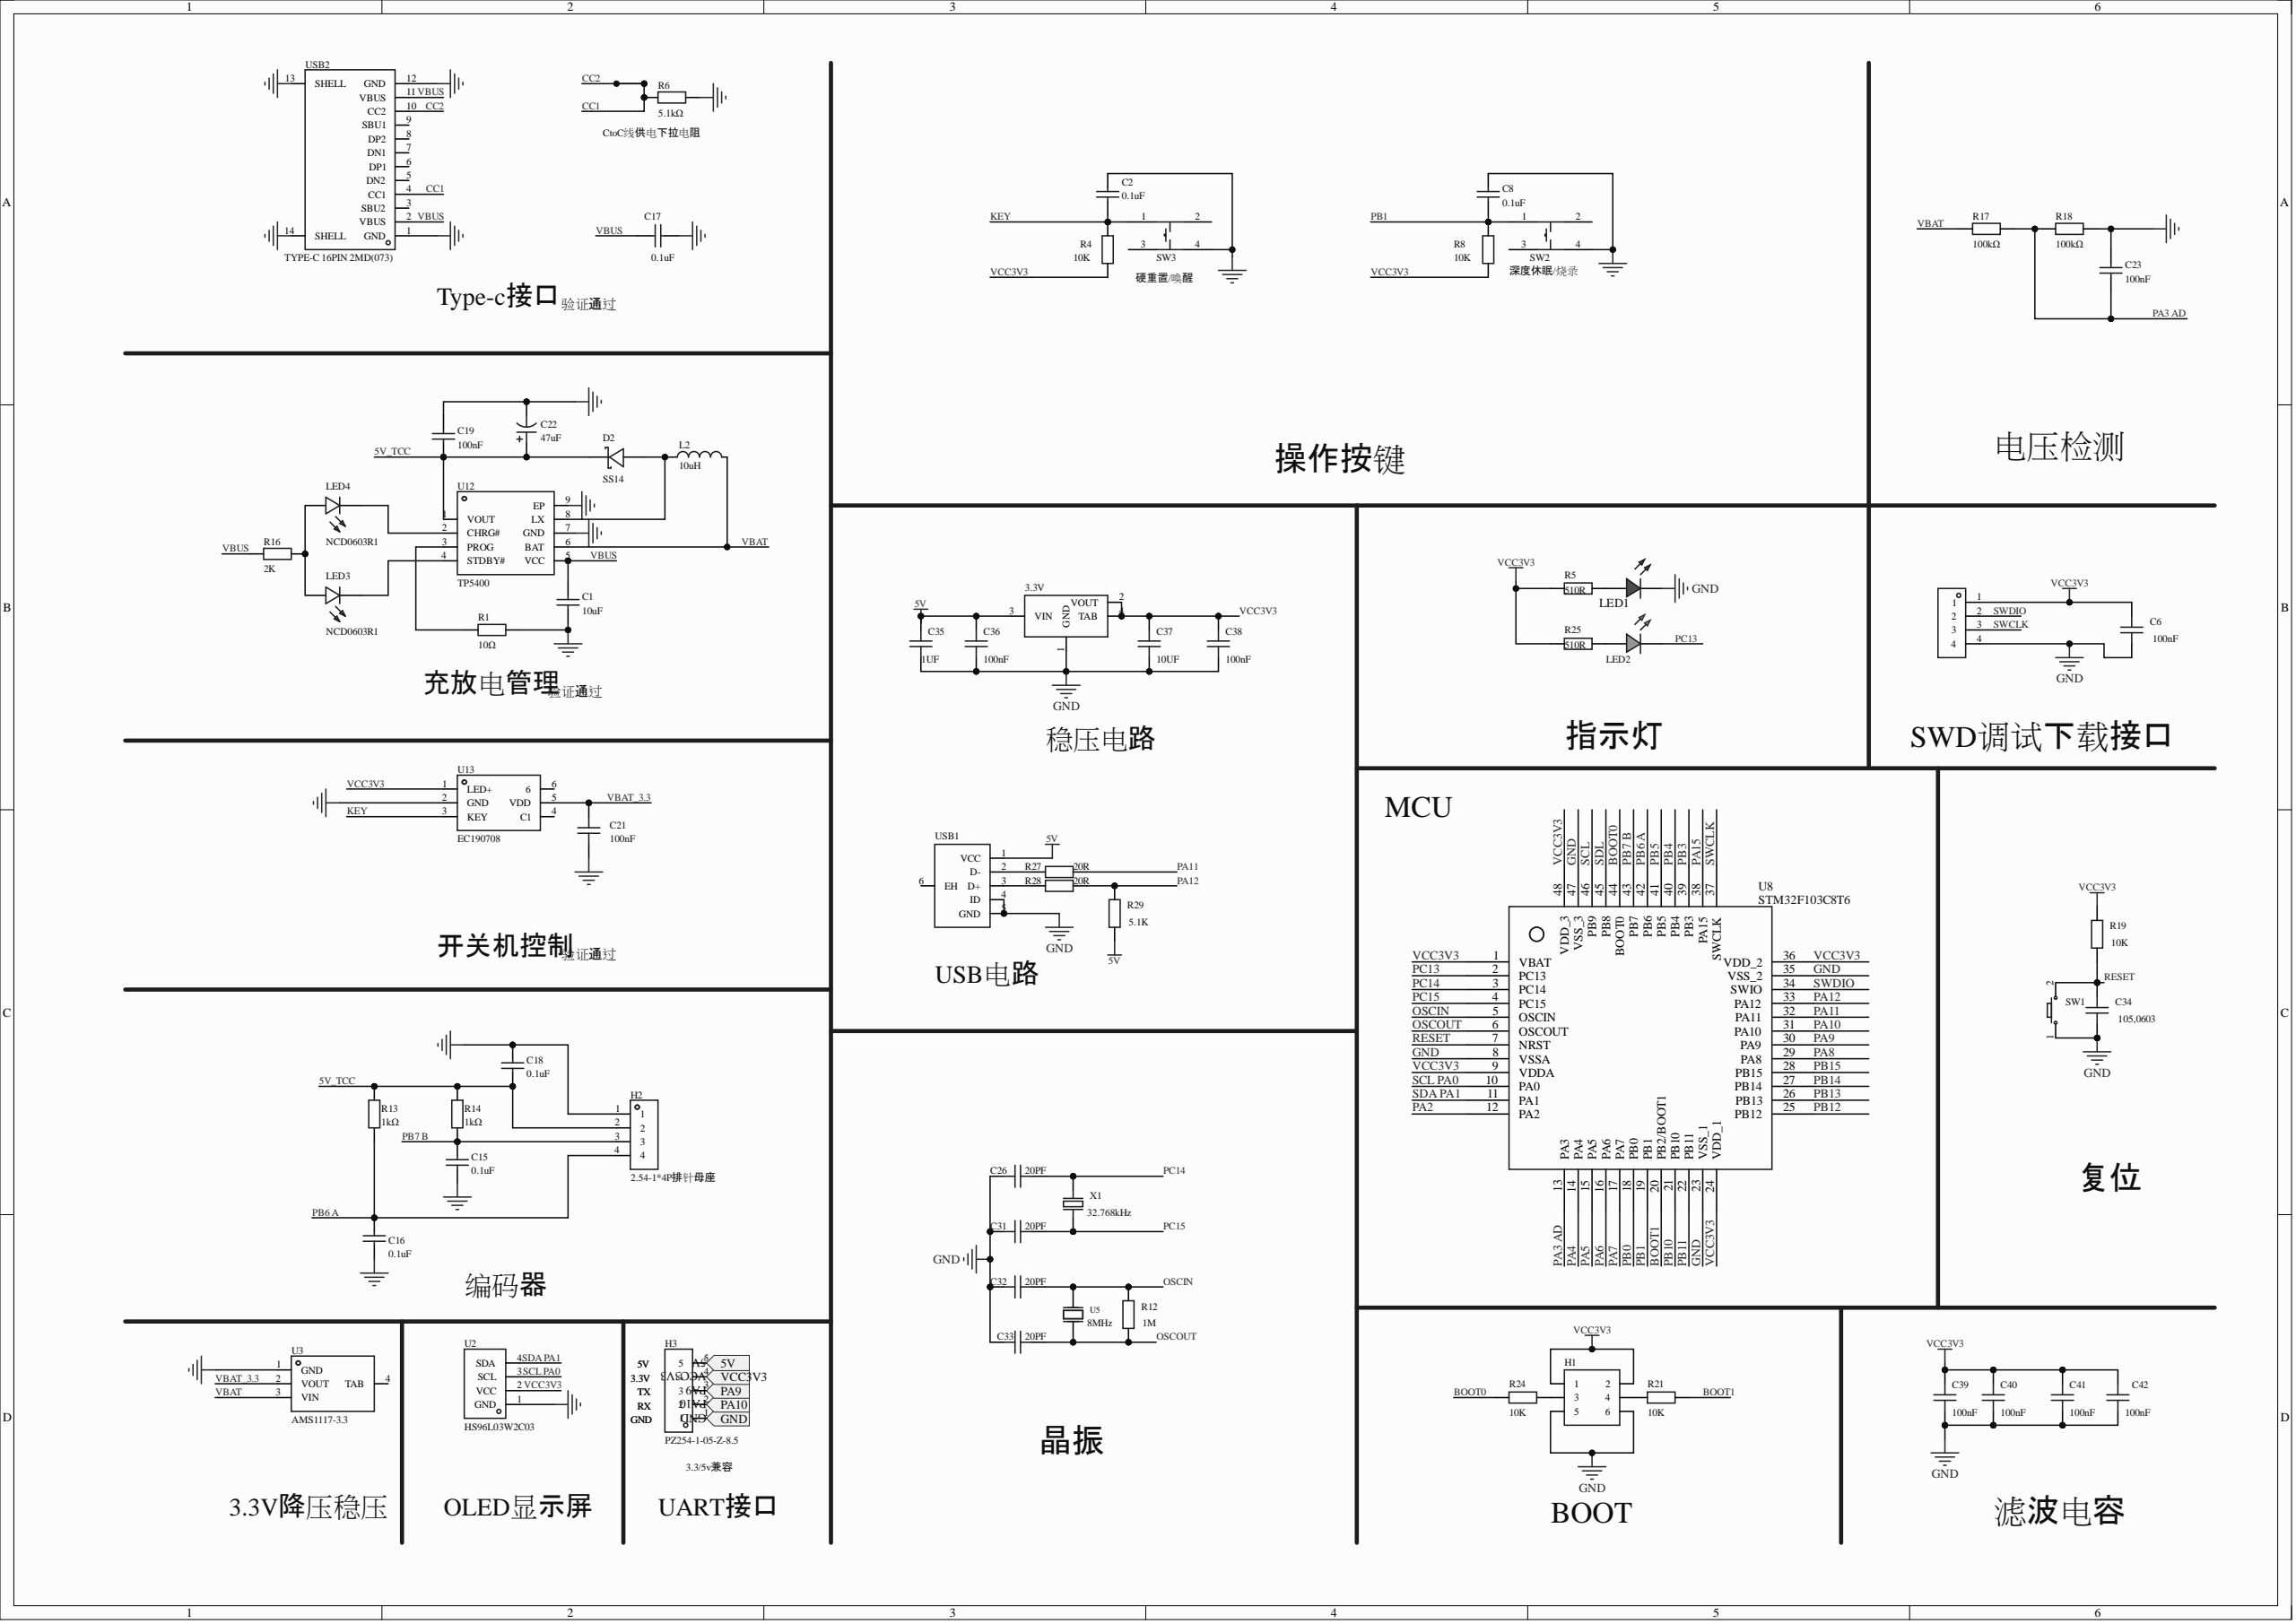Circuit board | Altium Designer | 66 parts | 40 nets
Bill of materials:
Comment,Description,Designator,Footprint,LibRef,Quantity
"","","3.3V","SOT_223","AMS1117","1"
"10uF","","C1, C37","C0805","CL21A106KAYNNNE_C15850, CAP_0805","2"
"0.1uF","","C2, C8, C15, C16, C17, C18","C0805","CL21A106KAYNNNE_C15850","6"
"100nF","","C6, C19, C23, C36, C38, C39, C40, C41, C42","C0805","CAP_0805, 0805B104K500NT","9"
"100nF","","C21","C0603","CC0603KRX7R9BB104","1"
"47uF","","C22","CAP-SMD_BD6.3-L6.6-W6.6-LS7.2-FD","RVT47UF35V67RV0039","1"
"20PF","","C26, C31, C32, C33","C0805","CAP_0805","4"
"105,0603","","C34","C0805","CAP_0805","1"
"1UF","","C35","C0805","CAP_0805","1"
"SS14","","D2","SMA_L4.2-W2.6-LS5.3-RD","SS14_C2480","1"
"","","H1","HDR-TH_6P-P2.54-V-R2-C3-S2.54_A2541WV-2X3P","HDR-M_2.54_2x3","1"
"2.54-1*4P排针母座","","H2","HDR-TH_4P-P2.54-V-F","2.54-1*4P母","1"
"PZ254-1-05-Z-8.5","","H3","HDR-TH_5P-P2.54-V-M","PZ254-1-05-Z-8.5","1"
"","","H5","HDR-TH_4P-P2.54-V-M","HDR-M_2.54_1x4P","1"
"10uH","","L2","IND-SMD_L7.3-W6.6","MCS0630-100MPY1","1"
"","","LED1, LED2","LED_0805","LED_0805-R, LED_0805-G","2"
"NCD0603R1","","LED3, LED4","LED0603-RD_RED","NCD0603R1_C84263","2"
"10Ω","","R1","R0805_NEW","Res_0603","1"
"10K","","R4, R8","R0805_NEW","Res_0603","2"
"510R","","R5, R25","R0805","Res_0805","2"
"5.1kΩ","","R6","R0805","0805W8F5101T5E","1"
"1M","","R12","R0805","Res_0805","1"
"1kΩ","","R13, R14","R0805","0805W8F1001T5E","2"
"2K","","R16","R0805_NEW","Res_0603","1"
"100kΩ","","R17, R18","R0805","0805W8F1003T5E","2"
"10K","","R19, R21, R24","R0805","Res_0805","3"
"20R","","R27, R28","R0805","Res_0805","2"
"5.1K","","R29","R0805","Res_0805","1"
"","","SW1","Key_SMD_3.6x6.1x2.5","Key_SMD_3.6x6.1x2.5","1"
"TS-1002S-13026C","","SW2, SW3","SW-SMD_4P-L6.0-W6.0-P4.50-LS9.0-2","TS-1002S-13026C","2"
"HS96L03W2C03","","U2","OLED-TH_L27.8-W27.2-P2.54_C9900033791","HS96L03W2C03","1"
"AMS1117-3.3","","U3","SOT-223-3_L6.5-W3.5-P3.05-LS7.0","AMS1117-3.3_C5250992","1"
"8MHz","","U5","CRYSTAL-TH_L10.8-W4.5-P4.88","ATS100B-E","1"
"STM32F103C8T6","","U8","LQFP-48_L7.0-W7.0-P0.50-LS9.0-BL","U2_STM32","1"
"TP5400","","U12","ESOP-8_L4.9-W3.9-P1.27-LS6.0-BL-EP","TP5400","1"
"EC190708","","U13","SOT-23-6_L2.9-W1.6-P0.95-LS2.8-BR","EC190708-15FF-1925","1"
"","","USB1","USB_Micro","USB_Micro-B","1"
"TYPE-C 16PIN 2MD(073)","","USB2","USB-C-SMD_TYPE-C-6PIN-2MD-073","TYPE-C 16PIN 2MD(073)","1"
"32.768kHz","","X1","FC-135R_L3.2-W1.5","Q13FC1350000400","1"
Netlist (Protel format):
[
3.3V
SOT_223




]
[
C1
C0805
10uF



]
[
C2
C0805
0.1uF



]
[
C6
C0805
100nF



]
[
C8
C0805
0.1uF



]
[
C15
C0805
0.1uF



]
[
C16
C0805
0.1uF



]
[
C17
C0805
0.1uF



]
[
C18
C0805
0.1uF



]
[
C19
C0805
100nF



]
[
C21
C0603
100nF



]
[
C22
CAP-SMD_BD6.3-L6.6-W6.6-LS7.2-FD
47uF



]
[
C23
C0805
100nF



]
[
C26
C0805
20PF



]
[
C31
C0805
20PF



]
[
C32
C0805
20PF



]
[
C33
C0805
20PF



]
[
C34
C0805
105,0603



]
[
C35
C0805
1UF



]
[
C36
C0805
100nF



]
[
C37
C0805
10UF



]
[
C38
C0805
100nF



]
[
C39
C0805
100nF



]
[
C40
C0805
100nF



]
[
C41
C0805
100nF



]
[
C42
C0805
100nF



]
[
D2
SMA_L4.2-W2.6-LS5.3-RD
SS14



]
[
H1
HDR-TH_6P-P2.54-V-R2-C3-S2.54_A2541WV-2X3P




]
[
H2
HDR-TH_4P-P2.54-V-F
2.54-1*4P排针母座



]
[
H3
HDR-TH_5P-P2.54-V-M
PZ254-1-05-Z-8.5



]
[
H5
HDR-TH_4P-P2.54-V-M




]
[
L2
IND-SMD_L7.3-W6.6
10uH



]
[
LED1
LED_0805




]
[
LED2
LED_0805




]
[
LED3
LED0603-RD_RED
NCD0603R1



]
[
LED4
LED0603-RD_RED
NCD0603R1



]
[
R1
R0805_NEW
10Ω



]
[
R4
R0805_NEW
10K



]
[
R5
R0805
510R



]
[
R6
R0805
5.1kΩ



]
[
R8
R0805_NEW
10K



]
[
R12
R0805
1M



]
[
R13
R0805
1kΩ



]
[
R14
R0805
1kΩ



]
[
R16
R0805_NEW
2K



]
[
R17
R0805
100kΩ



]
[
R18
R0805
100kΩ



]
[
R19
R0805
10K



]
[
R21
R0805
10K



]
[
R24
R0805
10K



]
[
R25
R0805
510R



]
[
R27
R0805
20R



]
[
R28
R0805
20R



]
[
R29
R0805
5.1K



]
[
SW1
Key_SMD_3.6x6.1x2.5




]
[
SW2
SW-SMD_4P-L6.0-W6.0-P4.50-LS9.0-2
TS-1002S-13026C



]
[
SW3
SW-SMD_4P-L6.0-W6.0-P4.50-LS9.0-2
TS-1002S-13026C



]
[
U2
OLED-TH_L27.8-W27.2-P2.54_C9900033791
HS96L03W2C03



]
[
U3
SOT-223-3_L6.5-W3.5-P3.05-LS7.0
AMS1117-3.3



]
[
U5
CRYSTAL-TH_L10.8-W4.5-P4.88
8MHz



]
[
U8
LQFP-48_L7.0-W7.0-P0.50-LS9.0-BL
STM32F103C8T6



]
[
U12
ESOP-8_L4.9-W3.9-P1.27-LS6.0-BL-EP
TP5400



]
[
U13
SOT-23-6_L2.9-W1.6-P0.95-LS2.8-BR
EC190708



]
[
USB1
USB_Micro




]
[
USB2
USB-C-SMD_TYPE-C-6PIN-2MD-073
TYPE-C 16PIN 2MD(073)



]
[
X1
FC-135R_L3.2-W1.5
32.768kHz



]
(
VCC3V3
3.3V-2
3.3V-4
C6-2
C37-2
C38-2
C39-2
C40-2
C41-2
C42-2
H1-1
H1-2
H3-4
H5-1
R4-2
R5-1
R8-2
R19-2
R25-1
U2-2
U8-1
U8-9
U8-24
U8-36
U8-48
U13-1
)
(
VBUS
C1-2
C17-2
R16-2
U12-5
USB2-2
USB2-11
)
(
VBAT_3.3
C21-2
U3-2
U13-5
)
(
VBAT
L2-2
R17-1
U3-3
U12-6
)
(
SWDIO
H5-2
U8-34
)
(
SWCLK
H5-3
U8-37
)
(
SDA PA1
U2-4
U8-11
)
(
SCL PA0
U2-3
U8-10
)
(
RESET
C34-2
R19-1
SW1-2
U8-7
)
(
PC15
C31-2
U8-4
X1-1
)
(
PC14
C26-1
U8-3
X1-2
)
(
PC13
LED2-1
U8-2
)
(
PB7 B
C15-2
H2-3
R14-1
U8-43
)
(
PB6 A
C16-2
H2-4
R13-1
U8-42
)
(
PB1
C8-1
R8-1
SW2-1
U8-19
)
(
PA12
R28-2
R29-2
U8-33
)
(
PA11
R27-2
U8-32
)
(
PA10
H3-2
U8-31
)
(
PA9
H3-3
U8-30
)
(
PA3 AD
C23-1
R17-2
R18-1
U8-13
)
(
OSCOUT
C33-1
R12-1
U5-1
U8-6
)
(
OSCIN
C32-1
R12-2
U5-2
U8-5
)
(
NetR28_1
R28-1
USB1-3
)
(
NetR27_1
R27-1
USB1-2
)
(
NetR1_2
R1-2
U12-3
)
(
NetLED4_1
LED4-1
U12-2
)
(
NetLED3_2
LED3-2
LED4-2
R16-1
)
(
NetLED3_1
LED3-1
U12-4
)
(
NetLED2_2
LED2-2
R25-2
)
(
NetLED1_2
LED1-2
R5-2
)
(
NetH1_4
H1-4
R21-1
)
(
NetH1_3
H1-3
R24-2
)
(
NetD2_2
D2-2
L2-1
U12-8
)
(
KEY
C2-1
R4-1
SW3-1
U13-3
)
(
GND
3.3V-1
C1-1
C2-2
C6-1
C8-2
C15-1
C16-1
C17-1
C18-2
C19-2
C21-1
C22-2
C23-2
C26-2
C31-1
C32-2
C33-2
C34-1
C35-1
C36-1
C37-1
C38-1
C39-1
C40-1
C41-1
C42-1
H1-5
H1-6
H2-1
H3-1
H5-4
LED1-1
R1-1
R6-2
R18-2
SW1-1
SW2-4
SW3-4
U2-1
U3-1
U8-8
U8-23
U8-35
U8-47
U12-7
U12-9
U13-2
USB1-4
USB1-5
USB2-1
USB2-12
USB2-13
USB2-14
)
(
CC1
R6-1
USB2-4
USB2-10
)
(
BOOT1
R21-2
U8-20
)
(
BOOT0
R24-1
U8-44
)
(
5V_TCC
C18-1
C19-1
C22-1
D2-1
H2-2
R13-2
R14-2
U12-1
)
(
5V
3.3V-3
C35-2
C36-2
H3-5
R29-1
USB1-1
)